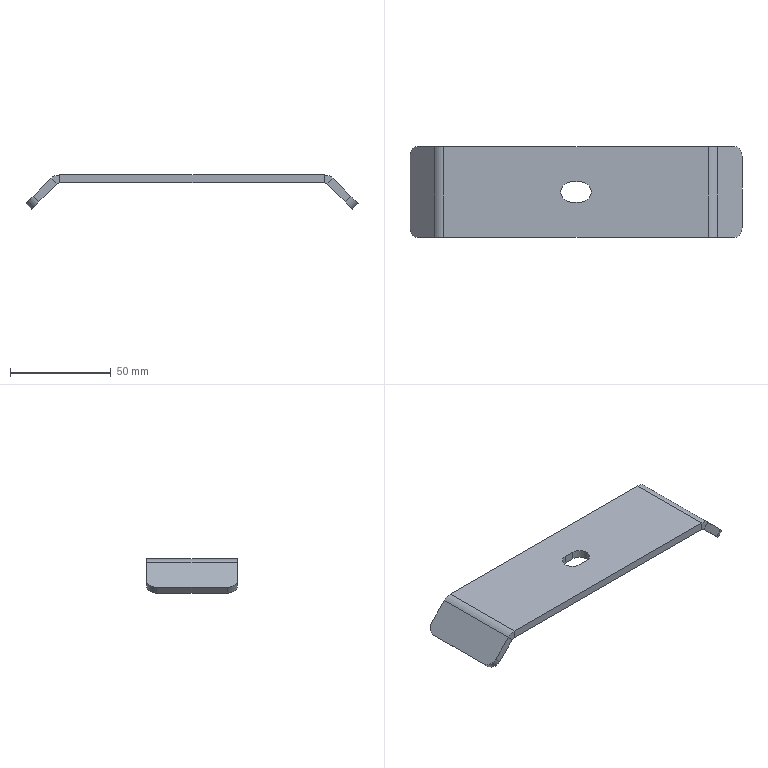Part | STEP file | PN_0074 guardrail connecting plate (spacing 120)_Default<As Machined> | 1 solid | 30 faces | box 164.912 x 45 x 17 mm | volume 30539 mm3 | plane 20 | cylinder 10 | commonest cylinder face diameters 10 x6 4 x2 12 x2